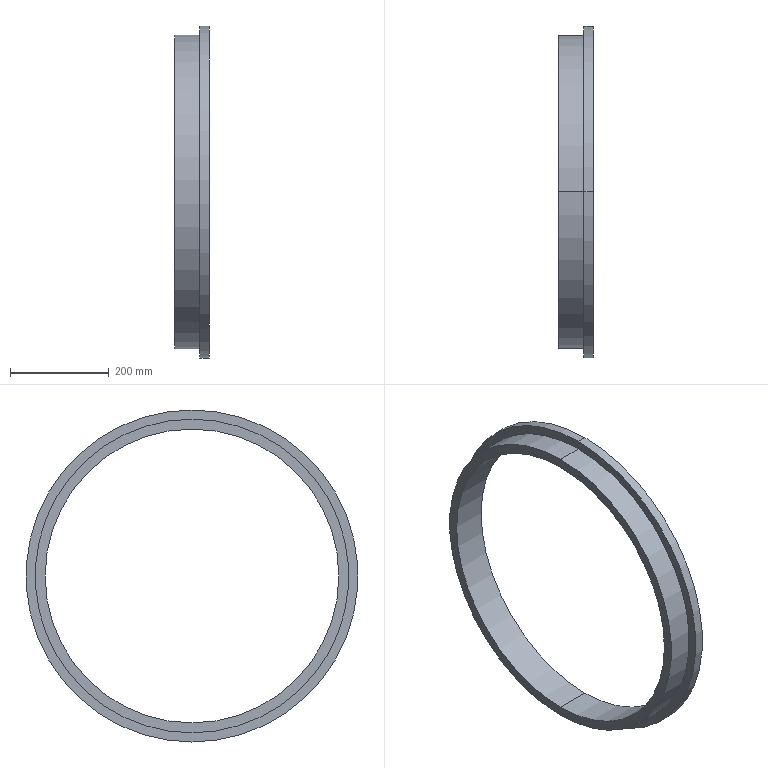Part | SolidWorks | features Revolution 1 | 1 solid | 9 faces | box 70 x 672.4 x 672.4 mm | volume 3434576 mm3 | cylinder 6 | plane 3 | commonest cylinder face diameters 595 x2 635 x2 672.4 x2
STEP:
#1=CARTESIAN_POINT('',(51.,0.,317.5));
#2=VERTEX_POINT('',#1);
#3=CARTESIAN_POINT('',(51.,0.,-317.5));
#4=VERTEX_POINT('',#3);
#5=CARTESIAN_POINT('',(51.,0.,0.));
#6=DIRECTION('',(-1.,0.,0.));
#7=DIRECTION('',(0.,0.,1.));
#8=AXIS2_PLACEMENT_3D('',#5,#6,#7);
#9=CIRCLE('',#8,317.5);
#10=EDGE_CURVE('',#2,#4,#9,.T.);
#11=ORIENTED_EDGE('',*,*,#10,.T.);
#12=CARTESIAN_POINT('',(0.,0.,-317.5));
#13=VERTEX_POINT('',#12);
#14=CARTESIAN_POINT('',(-185.132,0.,-317.5));
#15=DIRECTION('',(-1.,0.,0.));
#16=VECTOR('',#15,1000.);
#17=LINE('',#14,#16);
#18=EDGE_CURVE('',#4,#13,#17,.T.);
#19=ORIENTED_EDGE('',*,*,#18,.T.);
#20=CARTESIAN_POINT('',(0.,0.,317.5));
#21=VERTEX_POINT('',#20);
#22=CARTESIAN_POINT('',(0.,0.,0.));
#23=DIRECTION('',(-1.,0.,0.));
#24=DIRECTION('',(0.,0.,1.));
#25=AXIS2_PLACEMENT_3D('',#22,#23,#24);
#26=CIRCLE('',#25,317.5);
#27=EDGE_CURVE('',#21,#13,#26,.T.);
#28=ORIENTED_EDGE('',*,*,#27,.F.);
#29=CARTESIAN_POINT('',(-185.132,0.,317.5));
#30=DIRECTION('',(-1.,0.,0.));
#31=VECTOR('',#30,1000.);
#32=LINE('',#29,#31);
#33=EDGE_CURVE('',#2,#21,#32,.T.);
#34=ORIENTED_EDGE('',*,*,#33,.F.);
#35=EDGE_LOOP('',(#11,#19,#28,#34));
#36=FACE_OUTER_BOUND('',#35,.T.);
#37=CARTESIAN_POINT('',(-185.132,0.,0.));
#38=DIRECTION('',(-1.,0.,0.));
#39=DIRECTION('',(0.,0.,1.));
#40=AXIS2_PLACEMENT_3D('',#37,#38,#39);
#41=CYLINDRICAL_SURFACE('',#40,317.5);
#42=ADVANCED_FACE('',(#36),#41,.T.);
#43=CARTESIAN_POINT('',(70.,0.,336.2));
#44=VERTEX_POINT('',#43);
#45=CARTESIAN_POINT('',(70.,0.,-336.2));
#46=VERTEX_POINT('',#45);
#47=CARTESIAN_POINT('',(70.,0.,0.));
#48=DIRECTION('',(-1.,0.,0.));
#49=DIRECTION('',(0.,0.,1.));
#50=AXIS2_PLACEMENT_3D('',#47,#48,#49);
#51=CIRCLE('',#50,336.2);
#52=EDGE_CURVE('',#44,#46,#51,.T.);
#53=ORIENTED_EDGE('',*,*,#52,.T.);
#54=CARTESIAN_POINT('',(51.,0.,-336.2));
#55=VERTEX_POINT('',#54);
#56=CARTESIAN_POINT('',(-185.132,0.,-336.2));
#57=DIRECTION('',(-1.,0.,0.));
#58=VECTOR('',#57,1000.);
#59=LINE('',#56,#58);
#60=EDGE_CURVE('',#46,#55,#59,.T.);
#61=ORIENTED_EDGE('',*,*,#60,.T.);
#62=CARTESIAN_POINT('',(51.,0.,336.2));
#63=VERTEX_POINT('',#62);
#64=CARTESIAN_POINT('',(51.,0.,0.));
#65=DIRECTION('',(-1.,0.,0.));
#66=DIRECTION('',(0.,0.,1.));
#67=AXIS2_PLACEMENT_3D('',#64,#65,#66);
#68=CIRCLE('',#67,336.2);
#69=EDGE_CURVE('',#63,#55,#68,.T.);
#70=ORIENTED_EDGE('',*,*,#69,.F.);
#71=CARTESIAN_POINT('',(-185.132,0.,336.2));
#72=DIRECTION('',(-1.,0.,0.));
#73=VECTOR('',#72,1000.);
#74=LINE('',#71,#73);
#75=EDGE_CURVE('',#44,#63,#74,.T.);
#76=ORIENTED_EDGE('',*,*,#75,.F.);
#77=EDGE_LOOP('',(#53,#61,#70,#76));
#78=FACE_OUTER_BOUND('',#77,.T.);
#79=CARTESIAN_POINT('',(-185.132,0.,0.));
#80=DIRECTION('',(-1.,0.,0.));
#81=DIRECTION('',(0.,0.,1.));
#82=AXIS2_PLACEMENT_3D('',#79,#80,#81);
#83=CYLINDRICAL_SURFACE('',#82,336.2);
#84=ADVANCED_FACE('',(#78),#83,.T.);
#85=CARTESIAN_POINT('',(70.,0.,-297.5));
#86=VERTEX_POINT('',#85);
#87=CARTESIAN_POINT('',(70.,0.,297.5));
#88=VERTEX_POINT('',#87);
#89=CARTESIAN_POINT('',(70.,0.,0.));
#90=DIRECTION('',(-1.,0.,0.));
#91=DIRECTION('',(0.,0.,1.));
#92=AXIS2_PLACEMENT_3D('',#89,#90,#91);
#93=CIRCLE('',#92,297.5);
#94=EDGE_CURVE('',#86,#88,#93,.T.);
#95=ORIENTED_EDGE('',*,*,#94,.F.);
#96=CARTESIAN_POINT('',(0.,0.,-297.5));
#97=VERTEX_POINT('',#96);
#98=CARTESIAN_POINT('',(-185.132,0.,-297.5));
#99=DIRECTION('',(-1.,0.,0.));
#100=VECTOR('',#99,1000.);
#101=LINE('',#98,#100);
#102=EDGE_CURVE('',#86,#97,#101,.T.);
#103=ORIENTED_EDGE('',*,*,#102,.T.);
#104=CARTESIAN_POINT('',(0.,0.,297.5));
#105=VERTEX_POINT('',#104);
#106=CARTESIAN_POINT('',(0.,0.,0.));
#107=DIRECTION('',(-1.,0.,0.));
#108=DIRECTION('',(0.,0.,1.));
#109=AXIS2_PLACEMENT_3D('',#106,#107,#108);
#110=CIRCLE('',#109,297.5);
#111=EDGE_CURVE('',#97,#105,#110,.T.);
#112=ORIENTED_EDGE('',*,*,#111,.T.);
#113=CARTESIAN_POINT('',(-185.132,0.,297.5));
#114=DIRECTION('',(-1.,0.,0.));
#115=VECTOR('',#114,1000.);
#116=LINE('',#113,#115);
#117=EDGE_CURVE('',#88,#105,#116,.T.);
#118=ORIENTED_EDGE('',*,*,#117,.F.);
#119=EDGE_LOOP('',(#95,#103,#112,#118));
#120=FACE_OUTER_BOUND('',#119,.T.);
#121=CARTESIAN_POINT('',(-185.132,0.,0.));
#122=DIRECTION('',(-1.,0.,0.));
#123=DIRECTION('',(0.,0.,1.));
#124=AXIS2_PLACEMENT_3D('',#121,#122,#123);
#125=CYLINDRICAL_SURFACE('',#124,297.5);
#126=ADVANCED_FACE('',(#120),#125,.F.);
#127=CARTESIAN_POINT('',(0.,0.,0.));
#128=DIRECTION('',(-1.,0.,0.));
#129=DIRECTION('',(0.,0.,1.));
#130=AXIS2_PLACEMENT_3D('',#127,#128,#129);
#131=CIRCLE('',#130,297.5);
#132=EDGE_CURVE('',#105,#97,#131,.T.);
#133=ORIENTED_EDGE('',*,*,#132,.F.);
#134=ORIENTED_EDGE('',*,*,#111,.F.);
#135=EDGE_LOOP('',(#133,#134));
#136=FACE_BOUND('',#135,.T.);
#137=ORIENTED_EDGE('',*,*,#27,.T.);
#138=CARTESIAN_POINT('',(0.,0.,0.));
#139=DIRECTION('',(-1.,0.,0.));
#140=DIRECTION('',(0.,0.,1.));
#141=AXIS2_PLACEMENT_3D('',#138,#139,#140);
#142=CIRCLE('',#141,317.5);
#143=EDGE_CURVE('',#13,#21,#142,.T.);
#144=ORIENTED_EDGE('',*,*,#143,.T.);
#145=EDGE_LOOP('',(#137,#144));
#146=FACE_OUTER_BOUND('',#145,.T.);
#147=CARTESIAN_POINT('',(0.,317.5,0.));
#148=DIRECTION('',(1.,0.,0.));
#149=DIRECTION('',(0.,0.,-1.));
#150=AXIS2_PLACEMENT_3D('',#147,#148,#149);
#151=PLANE('',#150);
#152=ADVANCED_FACE('',(#136,#146),#151,.F.);
#153=ORIENTED_EDGE('',*,*,#102,.F.);
#154=CARTESIAN_POINT('',(70.,0.,0.));
#155=DIRECTION('',(-1.,0.,0.));
#156=DIRECTION('',(0.,0.,1.));
#157=AXIS2_PLACEMENT_3D('',#154,#155,#156);
#158=CIRCLE('',#157,297.5);
#159=EDGE_CURVE('',#88,#86,#158,.T.);
#160=ORIENTED_EDGE('',*,*,#159,.F.);
#161=ORIENTED_EDGE('',*,*,#117,.T.);
#162=ORIENTED_EDGE('',*,*,#132,.T.);
#163=EDGE_LOOP('',(#153,#160,#161,#162));
#164=FACE_OUTER_BOUND('',#163,.T.);
#165=CARTESIAN_POINT('',(-185.132,0.,0.));
#166=DIRECTION('',(-1.,0.,0.));
#167=DIRECTION('',(0.,0.,1.));
#168=AXIS2_PLACEMENT_3D('',#165,#166,#167);
#169=CYLINDRICAL_SURFACE('',#168,297.5);
#170=ADVANCED_FACE('',(#164),#169,.F.);
#171=ORIENTED_EDGE('',*,*,#52,.F.);
#172=CARTESIAN_POINT('',(70.,0.,0.));
#173=DIRECTION('',(-1.,0.,0.));
#174=DIRECTION('',(0.,0.,1.));
#175=AXIS2_PLACEMENT_3D('',#172,#173,#174);
#176=CIRCLE('',#175,336.2);
#177=EDGE_CURVE('',#46,#44,#176,.T.);
#178=ORIENTED_EDGE('',*,*,#177,.F.);
#179=EDGE_LOOP('',(#171,#178));
#180=FACE_OUTER_BOUND('',#179,.T.);
#181=ORIENTED_EDGE('',*,*,#159,.T.);
#182=ORIENTED_EDGE('',*,*,#94,.T.);
#183=EDGE_LOOP('',(#181,#182));
#184=FACE_BOUND('',#183,.T.);
#185=CARTESIAN_POINT('',(70.,297.5,0.));
#186=DIRECTION('',(-1.,0.,0.));
#187=DIRECTION('',(0.,0.,1.));
#188=AXIS2_PLACEMENT_3D('',#185,#186,#187);
#189=PLANE('',#188);
#190=ADVANCED_FACE('',(#180,#184),#189,.F.);
#191=ORIENTED_EDGE('',*,*,#60,.F.);
#192=ORIENTED_EDGE('',*,*,#177,.T.);
#193=ORIENTED_EDGE('',*,*,#75,.T.);
#194=CARTESIAN_POINT('',(51.,0.,0.));
#195=DIRECTION('',(-1.,0.,0.));
#196=DIRECTION('',(0.,0.,1.));
#197=AXIS2_PLACEMENT_3D('',#194,#195,#196);
#198=CIRCLE('',#197,336.2);
#199=EDGE_CURVE('',#55,#63,#198,.T.);
#200=ORIENTED_EDGE('',*,*,#199,.F.);
#201=EDGE_LOOP('',(#191,#192,#193,#200));
#202=FACE_OUTER_BOUND('',#201,.T.);
#203=CARTESIAN_POINT('',(-185.132,0.,0.));
#204=DIRECTION('',(-1.,0.,0.));
#205=DIRECTION('',(0.,0.,1.));
#206=AXIS2_PLACEMENT_3D('',#203,#204,#205);
#207=CYLINDRICAL_SURFACE('',#206,336.2);
#208=ADVANCED_FACE('',(#202),#207,.T.);
#209=ORIENTED_EDGE('',*,*,#10,.F.);
#210=CARTESIAN_POINT('',(51.,0.,0.));
#211=DIRECTION('',(-1.,0.,0.));
#212=DIRECTION('',(0.,0.,1.));
#213=AXIS2_PLACEMENT_3D('',#210,#211,#212);
#214=CIRCLE('',#213,317.5);
#215=EDGE_CURVE('',#4,#2,#214,.T.);
#216=ORIENTED_EDGE('',*,*,#215,.F.);
#217=EDGE_LOOP('',(#209,#216));
#218=FACE_BOUND('',#217,.T.);
#219=ORIENTED_EDGE('',*,*,#69,.T.);
#220=ORIENTED_EDGE('',*,*,#199,.T.);
#221=EDGE_LOOP('',(#219,#220));
#222=FACE_OUTER_BOUND('',#221,.T.);
#223=CARTESIAN_POINT('',(51.,336.2,0.));
#224=DIRECTION('',(1.,0.,0.));
#225=DIRECTION('',(0.,0.,-1.));
#226=AXIS2_PLACEMENT_3D('',#223,#224,#225);
#227=PLANE('',#226);
#228=ADVANCED_FACE('',(#218,#222),#227,.F.);
#229=ORIENTED_EDGE('',*,*,#18,.F.);
#230=ORIENTED_EDGE('',*,*,#215,.T.);
#231=ORIENTED_EDGE('',*,*,#33,.T.);
#232=ORIENTED_EDGE('',*,*,#143,.F.);
#233=EDGE_LOOP('',(#229,#230,#231,#232));
#234=FACE_OUTER_BOUND('',#233,.T.);
#235=CARTESIAN_POINT('',(-185.132,0.,0.));
#236=DIRECTION('',(-1.,0.,0.));
#237=DIRECTION('',(0.,0.,1.));
#238=AXIS2_PLACEMENT_3D('',#235,#236,#237);
#239=CYLINDRICAL_SURFACE('',#238,317.5);
#240=ADVANCED_FACE('',(#234),#239,.T.);
#241=CLOSED_SHELL('',(#42,#84,#126,#152,#170,#190,#208,#228,#240));
#242=MANIFOLD_SOLID_BREP('',#241);
#243=CARTESIAN_POINT('',(0.,0.,0.));
#244=DIRECTION('',(0.,0.,1.));
#245=DIRECTION('',(1.,0.,0.));
#246=AXIS2_PLACEMENT_3D('',#243,#244,#245);
#247=(LENGTH_UNIT()NAMED_UNIT(*)SI_UNIT(.MILLI.,.METRE.));
#248=UNCERTAINTY_MEASURE_WITH_UNIT(LENGTH_MEASURE(0.00001),#247,'','');
#249=(NAMED_UNIT(*)PLANE_ANGLE_UNIT()SI_UNIT($,.RADIAN.));
#250=(NAMED_UNIT(*)SI_UNIT($,.STERADIAN.)SOLID_ANGLE_UNIT());
#251=(GEOMETRIC_REPRESENTATION_CONTEXT(3)GLOBAL_UNCERTAINTY_ASSIGNED_CONTEXT((#248))GLOBAL_UNIT_ASSIGNED_CONTEXT((#247,#249,#250))REPRESENTATION_CONTEXT('',''));
#252=ADVANCED_BREP_SHAPE_REPRESENTATION('',(#242,#246),#251);